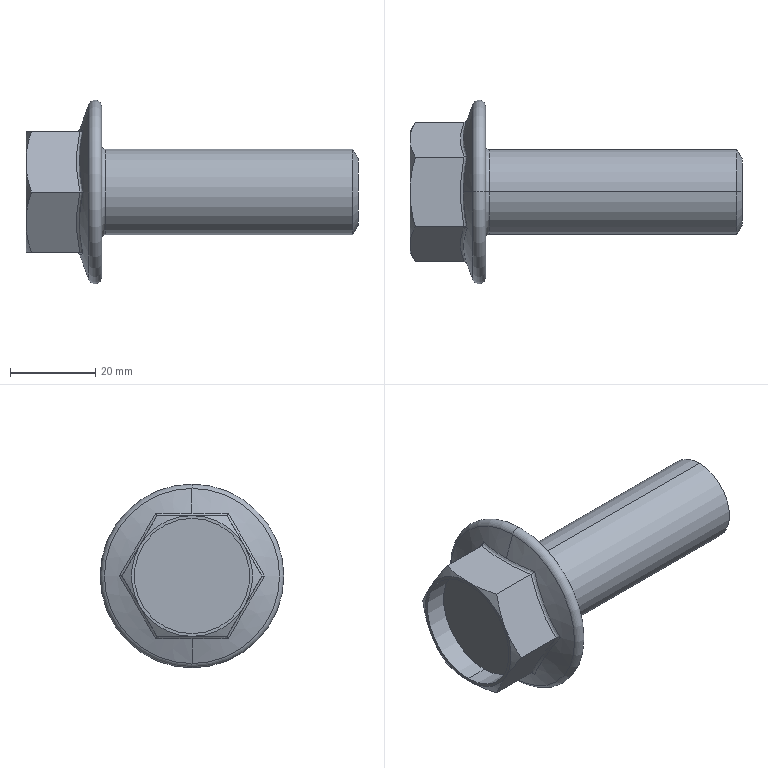Part | SolidWorks | 1 solid | 34 faces | box 77.7 x 43 x 43 mm | volume 30766 mm3 | cone 10 | plane 10 | spline 6 | torus 4 | cylinder 4 | commonest cylinder face diameters 20 x2 27 x2
STEP:
#1=CARTESIAN_POINT('',(0.,0.,-10.8));
#2=VERTEX_POINT('',#1);
#3=CARTESIAN_POINT('',(0.,0.,10.8));
#4=VERTEX_POINT('',#3);
#5=CARTESIAN_POINT('',(0.,0.,0.));
#6=DIRECTION('',(-1.,0.,0.));
#7=DIRECTION('',(0.,0.,1.));
#8=AXIS2_PLACEMENT_3D('',#5,#6,#7);
#9=CIRCLE('',#8,10.8);
#10=EDGE_CURVE('',#2,#4,#9,.T.);
#11=ORIENTED_EDGE('',*,*,#10,.F.);
#12=CARTESIAN_POINT('',(0.8,0.,-10.));
#13=VERTEX_POINT('',#12);
#14=CARTESIAN_POINT('',(0.8,0.,-10.8));
#15=DIRECTION('',(0.,1.,0.));
#16=DIRECTION('',(0.,0.,1.));
#17=AXIS2_PLACEMENT_3D('',#14,#15,#16);
#18=CIRCLE('',#17,0.8);
#19=EDGE_CURVE('',#2,#13,#18,.T.);
#20=ORIENTED_EDGE('',*,*,#19,.T.);
#21=CARTESIAN_POINT('',(0.8,0.,10.));
#22=VERTEX_POINT('',#21);
#23=CARTESIAN_POINT('',(0.8,0.,0.));
#24=DIRECTION('',(1.,0.,0.));
#25=DIRECTION('',(0.,0.,1.));
#26=AXIS2_PLACEMENT_3D('',#23,#24,#25);
#27=CIRCLE('',#26,10.);
#28=EDGE_CURVE('',#22,#13,#27,.T.);
#29=ORIENTED_EDGE('',*,*,#28,.F.);
#30=CARTESIAN_POINT('',(0.8,0.,10.8));
#31=DIRECTION('',(0.,-1.,0.));
#32=DIRECTION('',(0.,0.,-1.));
#33=AXIS2_PLACEMENT_3D('',#30,#31,#32);
#34=CIRCLE('',#33,0.8);
#35=EDGE_CURVE('',#4,#22,#34,.T.);
#36=ORIENTED_EDGE('',*,*,#35,.F.);
#37=EDGE_LOOP('',(#11,#20,#29,#36));
#38=FACE_OUTER_BOUND('',#37,.T.);
#39=CARTESIAN_POINT('',(0.8,0.,0.));
#40=DIRECTION('',(-1.,0.,0.));
#41=DIRECTION('',(0.,0.,1.));
#42=AXIS2_PLACEMENT_3D('',#39,#40,#41);
#43=TOROIDAL_SURFACE('',#42,10.8,0.8);
#44=ADVANCED_FACE('',(#38),#43,.F.);
#45=CARTESIAN_POINT('',(60.,0.,7.835));
#46=VERTEX_POINT('',#45);
#47=CARTESIAN_POINT('',(60.,0.,-7.835));
#48=VERTEX_POINT('',#47);
#49=CARTESIAN_POINT('',(60.,0.,0.));
#50=DIRECTION('',(-1.,0.,0.));
#51=DIRECTION('',(0.,0.,1.));
#52=AXIS2_PLACEMENT_3D('',#49,#50,#51);
#53=CIRCLE('',#52,7.835);
#54=EDGE_CURVE('',#46,#48,#53,.T.);
#55=ORIENTED_EDGE('',*,*,#54,.T.);
#56=CARTESIAN_POINT('',(58.75,0.,-10.));
#57=VERTEX_POINT('',#56);
#58=CARTESIAN_POINT('',(58.75,0.,-10.));
#59=DIRECTION('',(-0.5,0.,-0.866));
#60=VECTOR('',#59,1000.);
#61=LINE('',#58,#60);
#62=EDGE_CURVE('',#48,#57,#61,.T.);
#63=ORIENTED_EDGE('',*,*,#62,.T.);
#64=CARTESIAN_POINT('',(58.75,0.,10.));
#65=VERTEX_POINT('',#64);
#66=CARTESIAN_POINT('',(58.75,0.,0.));
#67=DIRECTION('',(-1.,0.,0.));
#68=DIRECTION('',(0.,0.,1.));
#69=AXIS2_PLACEMENT_3D('',#66,#67,#68);
#70=CIRCLE('',#69,10.);
#71=EDGE_CURVE('',#65,#57,#70,.T.);
#72=ORIENTED_EDGE('',*,*,#71,.F.);
#73=CARTESIAN_POINT('',(58.75,0.,10.));
#74=DIRECTION('',(-0.5,0.,0.866));
#75=VECTOR('',#74,1000.);
#76=LINE('',#73,#75);
#77=EDGE_CURVE('',#46,#65,#76,.T.);
#78=ORIENTED_EDGE('',*,*,#77,.F.);
#79=EDGE_LOOP('',(#55,#63,#72,#78));
#80=FACE_OUTER_BOUND('',#79,.T.);
#81=CARTESIAN_POINT('',(58.75,0.,0.));
#82=DIRECTION('',(-1.,0.,0.));
#83=DIRECTION('',(0.,0.,1.));
#84=AXIS2_PLACEMENT_3D('',#81,#82,#83);
#85=CONICAL_SURFACE('',#84,10.,1.047);
#86=ADVANCED_FACE('',(#80),#85,.T.);
#87=CARTESIAN_POINT('',(-12.411,0.,-13.5));
#88=VERTEX_POINT('',#87);
#89=CARTESIAN_POINT('',(-12.411,0.,13.5));
#90=VERTEX_POINT('',#89);
#91=CARTESIAN_POINT('',(-12.411,0.,0.));
#92=DIRECTION('',(-1.,0.,0.));
#93=DIRECTION('',(0.,0.,1.));
#94=AXIS2_PLACEMENT_3D('',#91,#92,#93);
#95=CIRCLE('',#94,13.5);
#96=EDGE_CURVE('',#88,#90,#95,.T.);
#97=ORIENTED_EDGE('',*,*,#96,.F.);
#98=CARTESIAN_POINT('',(-17.7,0.,-13.5));
#99=VERTEX_POINT('',#98);
#100=CARTESIAN_POINT('',(-12.411,0.,-13.5));
#101=DIRECTION('',(-1.,0.,0.));
#102=VECTOR('',#101,1000.);
#103=LINE('',#100,#102);
#104=EDGE_CURVE('',#88,#99,#103,.T.);
#105=ORIENTED_EDGE('',*,*,#104,.T.);
#106=CARTESIAN_POINT('',(-17.7,0.,13.5));
#107=VERTEX_POINT('',#106);
#108=CARTESIAN_POINT('',(-17.7,0.,0.));
#109=DIRECTION('',(-1.,0.,0.));
#110=DIRECTION('',(0.,0.,1.));
#111=AXIS2_PLACEMENT_3D('',#108,#109,#110);
#112=CIRCLE('',#111,13.5);
#113=EDGE_CURVE('',#99,#107,#112,.T.);
#114=ORIENTED_EDGE('',*,*,#113,.T.);
#115=CARTESIAN_POINT('',(-12.411,0.,13.5));
#116=DIRECTION('',(-1.,0.,0.));
#117=VECTOR('',#116,1000.);
#118=LINE('',#115,#117);
#119=EDGE_CURVE('',#90,#107,#118,.T.);
#120=ORIENTED_EDGE('',*,*,#119,.F.);
#121=EDGE_LOOP('',(#97,#105,#114,#120));
#122=FACE_OUTER_BOUND('',#121,.T.);
#123=CARTESIAN_POINT('',(-12.411,0.,0.));
#124=DIRECTION('',(-1.,0.,0.));
#125=DIRECTION('',(0.,0.,1.));
#126=AXIS2_PLACEMENT_3D('',#123,#124,#125);
#127=CYLINDRICAL_SURFACE('',#126,13.5);
#128=ADVANCED_FACE('',(#122),#127,.F.);
#129=CARTESIAN_POINT('',(0.,0.,19.953));
#130=VERTEX_POINT('',#129);
#131=CARTESIAN_POINT('',(0.,0.,-19.953));
#132=VERTEX_POINT('',#131);
#133=CARTESIAN_POINT('',(0.,0.,0.));
#134=DIRECTION('',(-1.,0.,0.));
#135=DIRECTION('',(0.,0.,1.));
#136=AXIS2_PLACEMENT_3D('',#133,#134,#135);
#137=CIRCLE('',#136,19.953);
#138=EDGE_CURVE('',#130,#132,#137,.T.);
#139=ORIENTED_EDGE('',*,*,#138,.T.);
#140=CARTESIAN_POINT('',(-3.,0.,-20.482));
#141=VERTEX_POINT('',#140);
#142=CARTESIAN_POINT('',(-1.547,0.,-19.953));
#143=DIRECTION('',(0.,1.,0.));
#144=DIRECTION('',(0.,0.,1.));
#145=AXIS2_PLACEMENT_3D('',#142,#143,#144);
#146=CIRCLE('',#145,1.547);
#147=EDGE_CURVE('',#132,#141,#146,.T.);
#148=ORIENTED_EDGE('',*,*,#147,.T.);
#149=CARTESIAN_POINT('',(-3.,0.,20.482));
#150=VERTEX_POINT('',#149);
#151=CARTESIAN_POINT('',(-3.,0.,0.));
#152=DIRECTION('',(-1.,0.,0.));
#153=DIRECTION('',(0.,0.,1.));
#154=AXIS2_PLACEMENT_3D('',#151,#152,#153);
#155=CIRCLE('',#154,20.482);
#156=EDGE_CURVE('',#150,#141,#155,.T.);
#157=ORIENTED_EDGE('',*,*,#156,.F.);
#158=CARTESIAN_POINT('',(-1.547,0.,19.953));
#159=DIRECTION('',(0.,-1.,0.));
#160=DIRECTION('',(0.,0.,-1.));
#161=AXIS2_PLACEMENT_3D('',#158,#159,#160);
#162=CIRCLE('',#161,1.547);
#163=EDGE_CURVE('',#130,#150,#162,.T.);
#164=ORIENTED_EDGE('',*,*,#163,.F.);
#165=EDGE_LOOP('',(#139,#148,#157,#164));
#166=FACE_OUTER_BOUND('',#165,.T.);
#167=CARTESIAN_POINT('',(-1.547,0.,0.));
#168=DIRECTION('',(-1.,0.,0.));
#169=DIRECTION('',(0.,0.,1.));
#170=AXIS2_PLACEMENT_3D('',#167,#168,#169);
#171=TOROIDAL_SURFACE('',#170,19.953,1.547);
#172=ADVANCED_FACE('',(#166),#171,.T.);
#173=CARTESIAN_POINT('',(-4.275,8.49,14.705));
#174=VERTEX_POINT('',#173);
#175=CARTESIAN_POINT('',(-5.116,0.,14.669));
#176=VERTEX_POINT('',#175);
#177=CARTESIAN_POINT('',(-4.275,8.49,14.705));
#178=CARTESIAN_POINT('',(-4.533,7.087,14.695));
#179=CARTESIAN_POINT('',(-4.745,5.679,14.686));
#180=CARTESIAN_POINT('',(-5.037,2.85,14.673));
#181=CARTESIAN_POINT('',(-5.116,1.429,14.669));
#182=CARTESIAN_POINT('',(-5.116,0.,14.669));
#183=B_SPLINE_CURVE_WITH_KNOTS('',3,(#177,#178,#179,#180,#181,#182),.UNSPECIFIED.,.F.,.F.,(4,2,4),(0.,0.004266,0.008532),.UNSPECIFIED.);
#184=EDGE_CURVE('',#174,#176,#183,.T.);
#185=ORIENTED_EDGE('',*,*,#184,.T.);
#186=CARTESIAN_POINT('',(-3.,0.,20.482));
#187=DIRECTION('',(0.342,0.,0.9397));
#188=VECTOR('',#187,1000.);
#189=LINE('',#186,#188);
#190=EDGE_CURVE('',#176,#150,#189,.T.);
#191=ORIENTED_EDGE('',*,*,#190,.T.);
#192=ORIENTED_EDGE('',*,*,#156,.T.);
#193=CARTESIAN_POINT('',(-5.116,0.,-14.669));
#194=VERTEX_POINT('',#193);
#195=CARTESIAN_POINT('',(-3.,0.,-20.482));
#196=DIRECTION('',(0.342,0.,-0.9397));
#197=VECTOR('',#196,1000.);
#198=LINE('',#195,#197);
#199=EDGE_CURVE('',#194,#141,#198,.T.);
#200=ORIENTED_EDGE('',*,*,#199,.F.);
#201=CARTESIAN_POINT('',(-4.275,8.49,-14.705));
#202=VERTEX_POINT('',#201);
#203=CARTESIAN_POINT('',(-5.116,0.,-14.669));
#204=CARTESIAN_POINT('',(-5.116,1.425,-14.669));
#205=CARTESIAN_POINT('',(-5.037,2.85,-14.673));
#206=CARTESIAN_POINT('',(-4.745,5.682,-14.686));
#207=CARTESIAN_POINT('',(-4.533,7.089,-14.695));
#208=CARTESIAN_POINT('',(-4.275,8.49,-14.705));
#209=B_SPLINE_CURVE_WITH_KNOTS('',3,(#203,#204,#205,#206,#207,#208),.UNSPECIFIED.,.F.,.F.,(4,2,4),(0.008532,0.01279,0.01704),.UNSPECIFIED.);
#210=EDGE_CURVE('',#194,#202,#209,.T.);
#211=ORIENTED_EDGE('',*,*,#210,.T.);
#212=CARTESIAN_POINT('',(-4.275,16.98,0.));
#213=VERTEX_POINT('',#212);
#214=CARTESIAN_POINT('',(-4.275,8.49,-14.705));
#215=CARTESIAN_POINT('',(-4.533,9.182,-13.487));
#216=CARTESIAN_POINT('',(-4.745,9.877,-12.264));
#217=CARTESIAN_POINT('',(-5.037,11.278,-9.811));
#218=CARTESIAN_POINT('',(-5.116,11.984,-8.579));
#219=CARTESIAN_POINT('',(-5.116,13.412,-6.108));
#220=CARTESIAN_POINT('',(-5.038,14.128,-4.874));
#221=CARTESIAN_POINT('',(-4.745,15.558,-2.426));
#222=CARTESIAN_POINT('',(-4.533,16.27,-1.21));
#223=CARTESIAN_POINT('',(-4.275,16.98,0.));
#224=B_SPLINE_CURVE_WITH_KNOTS('',3,(#214,#215,#216,#217,#218,#219,#220,#221,#222,#223),.UNSPECIFIED.,.F.,.F.,(4,2,2,2,4),(0.,0.004261,0.008521,0.01278,0.01704),.UNSPECIFIED.);
#225=EDGE_CURVE('',#202,#213,#224,.T.);
#226=ORIENTED_EDGE('',*,*,#225,.T.);
#227=CARTESIAN_POINT('',(-4.275,16.98,0.));
#228=CARTESIAN_POINT('',(-4.533,16.271,1.209));
#229=CARTESIAN_POINT('',(-4.745,15.56,2.422));
#230=CARTESIAN_POINT('',(-5.037,14.135,4.862));
#231=CARTESIAN_POINT('',(-5.116,13.422,6.089));
#232=CARTESIAN_POINT('',(-5.116,11.995,8.561));
#233=CARTESIAN_POINT('',(-5.038,11.285,9.798));
#234=CARTESIAN_POINT('',(-4.745,9.879,12.261));
#235=CARTESIAN_POINT('',(-4.533,9.183,13.485));
#236=CARTESIAN_POINT('',(-4.275,8.49,14.705));
#237=B_SPLINE_CURVE_WITH_KNOTS('',3,(#227,#228,#229,#230,#231,#232,#233,#234,#235,#236),.UNSPECIFIED.,.F.,.F.,(4,2,2,2,4),(0.,0.004261,0.008521,0.01278,0.01704),.UNSPECIFIED.);
#238=EDGE_CURVE('',#213,#174,#237,.T.);
#239=ORIENTED_EDGE('',*,*,#238,.T.);
#240=EDGE_LOOP('',(#185,#191,#192,#200,#211,#226,#239));
#241=FACE_OUTER_BOUND('',#240,.T.);
#242=CARTESIAN_POINT('',(-3.,0.,0.));
#243=DIRECTION('',(1.,0.,0.));
#244=DIRECTION('',(0.,0.,-1.));
#245=AXIS2_PLACEMENT_3D('',#242,#243,#244);
#246=CONICAL_SURFACE('',#245,20.482,1.222);
#247=ADVANCED_FACE('',(#241),#246,.T.);
#248=ORIENTED_EDGE('',*,*,#71,.T.);
#249=CARTESIAN_POINT('',(60.,0.,-10.));
#250=DIRECTION('',(-1.,0.,0.));
#251=VECTOR('',#250,1000.);
#252=LINE('',#249,#251);
#253=EDGE_CURVE('',#57,#13,#252,.T.);
#254=ORIENTED_EDGE('',*,*,#253,.T.);
#255=CARTESIAN_POINT('',(0.8,0.,0.));
#256=DIRECTION('',(1.,0.,0.));
#257=DIRECTION('',(0.,0.,1.));
#258=AXIS2_PLACEMENT_3D('',#255,#256,#257);
#259=CIRCLE('',#258,10.);
#260=EDGE_CURVE('',#13,#22,#259,.T.);
#261=ORIENTED_EDGE('',*,*,#260,.T.);
#262=CARTESIAN_POINT('',(60.,0.,10.));
#263=DIRECTION('',(-1.,0.,0.));
#264=VECTOR('',#263,1000.);
#265=LINE('',#262,#264);
#266=EDGE_CURVE('',#65,#22,#265,.T.);
#267=ORIENTED_EDGE('',*,*,#266,.F.);
#268=EDGE_LOOP('',(#248,#254,#261,#267));
#269=FACE_OUTER_BOUND('',#268,.T.);
#270=CARTESIAN_POINT('',(60.,0.,0.));
#271=DIRECTION('',(-1.,0.,0.));
#272=DIRECTION('',(0.,0.,1.));
#273=AXIS2_PLACEMENT_3D('',#270,#271,#272);
#274=CYLINDRICAL_SURFACE('',#273,10.);
#275=ADVANCED_FACE('',(#269),#274,.T.);
#276=ORIENTED_EDGE('',*,*,#253,.F.);
#277=CARTESIAN_POINT('',(58.75,0.,0.));
#278=DIRECTION('',(-1.,0.,0.));
#279=DIRECTION('',(0.,0.,1.));
#280=AXIS2_PLACEMENT_3D('',#277,#278,#279);
#281=CIRCLE('',#280,10.);
#282=EDGE_CURVE('',#57,#65,#281,.T.);
#283=ORIENTED_EDGE('',*,*,#282,.T.);
#284=ORIENTED_EDGE('',*,*,#266,.T.);
#285=ORIENTED_EDGE('',*,*,#28,.T.);
#286=EDGE_LOOP('',(#276,#283,#284,#285));
#287=FACE_OUTER_BOUND('',#286,.T.);
#288=CARTESIAN_POINT('',(60.,0.,0.));
#289=DIRECTION('',(-1.,0.,0.));
#290=DIRECTION('',(0.,0.,1.));
#291=AXIS2_PLACEMENT_3D('',#288,#289,#290);
#292=CYLINDRICAL_SURFACE('',#291,10.);
#293=ADVANCED_FACE('',(#287),#292,.T.);
#294=CARTESIAN_POINT('',(0.,0.,0.));
#295=DIRECTION('',(-1.,0.,0.));
#296=DIRECTION('',(0.,0.,1.));
#297=AXIS2_PLACEMENT_3D('',#294,#295,#296);
#298=CIRCLE('',#297,10.8);
#299=EDGE_CURVE('',#4,#2,#298,.T.);
#300=ORIENTED_EDGE('',*,*,#299,.T.);
#301=ORIENTED_EDGE('',*,*,#10,.T.);
#302=EDGE_LOOP('',(#300,#301));
#303=FACE_BOUND('',#302,.T.);
#304=ORIENTED_EDGE('',*,*,#138,.F.);
#305=CARTESIAN_POINT('',(0.,0.,0.));
#306=DIRECTION('',(-1.,0.,0.));
#307=DIRECTION('',(0.,0.,1.));
#308=AXIS2_PLACEMENT_3D('',#305,#306,#307);
#309=CIRCLE('',#308,19.953);
#310=EDGE_CURVE('',#132,#130,#309,.T.);
#311=ORIENTED_EDGE('',*,*,#310,.F.);
#312=EDGE_LOOP('',(#304,#311));
#313=FACE_OUTER_BOUND('',#312,.T.);
#314=CARTESIAN_POINT('',(0.,0.,0.));
#315=DIRECTION('',(-1.,0.,0.));
#316=DIRECTION('',(0.,0.,1.));
#317=AXIS2_PLACEMENT_3D('',#314,#315,#316);
#318=PLANE('',#317);
#319=ADVANCED_FACE('',(#303,#313),#318,.F.);
#320=CARTESIAN_POINT('',(-16.437,8.165,14.142));
#321=VERTEX_POINT('',#320);
#322=CARTESIAN_POINT('',(-5.109,8.165,14.142));
#323=VERTEX_POINT('',#322);
#324=CARTESIAN_POINT('',(-17.7,8.165,14.142));
#325=DIRECTION('',(1.,0.,0.));
#326=VECTOR('',#325,1000.);
#327=LINE('',#324,#326);
#328=EDGE_CURVE('',#321,#323,#327,.T.);
#329=ORIENTED_EDGE('',*,*,#328,.T.);
#330=CARTESIAN_POINT('',(-5.109,16.33,0.));
#331=VERTEX_POINT('',#330);
#332=CARTESIAN_POINT('',(-5.109,8.165,14.142));
#333=CARTESIAN_POINT('',(-5.345,8.84,12.972));
#334=CARTESIAN_POINT('',(-5.536,9.518,11.799));
#335=CARTESIAN_POINT('',(-5.798,10.878,9.443));
#336=CARTESIAN_POINT('',(-5.868,11.561,8.26));
#337=CARTESIAN_POINT('',(-5.868,12.934,5.882));
#338=CARTESIAN_POINT('',(-5.798,13.617,4.699));
#339=CARTESIAN_POINT('',(-5.536,14.977,2.343));
#340=CARTESIAN_POINT('',(-5.345,15.655,1.17));
#341=CARTESIAN_POINT('',(-5.109,16.33,0.));
#342=B_SPLINE_CURVE_WITH_KNOTS('',3,(#332,#333,#334,#335,#336,#337,#338,#339,#340,#341),.UNSPECIFIED.,.F.,.F.,(4,2,2,2,4),(0.,0.0041,0.0082,0.0123,0.0164),.UNSPECIFIED.);
#343=EDGE_CURVE('',#323,#331,#342,.T.);
#344=ORIENTED_EDGE('',*,*,#343,.T.);
#345=CARTESIAN_POINT('',(-16.437,16.33,0.));
#346=VERTEX_POINT('',#345);
#347=CARTESIAN_POINT('',(-17.7,16.33,0.));
#348=DIRECTION('',(1.,0.,0.));
#349=VECTOR('',#348,1000.);
#350=LINE('',#347,#349);
#351=EDGE_CURVE('',#346,#331,#350,.T.);
#352=ORIENTED_EDGE('',*,*,#351,.F.);
#353=CARTESIAN_POINT('',(-17.7,12.247,7.071));
#354=VERTEX_POINT('',#353);
#355=CARTESIAN_POINT('',(-17.7,12.247,7.071));
#356=CARTESIAN_POINT('',(-17.7,12.594,6.471));
#357=CARTESIAN_POINT('',(-17.67,12.942,5.868));
#358=CARTESIAN_POINT('',(-17.555,13.63,4.676));
#359=CARTESIAN_POINT('',(-17.469,13.972,4.084));
#360=CARTESIAN_POINT('',(-17.139,14.992,2.317));
#361=CARTESIAN_POINT('',(-16.821,15.664,1.154));
#362=CARTESIAN_POINT('',(-16.437,16.33,0.));
#363=B_SPLINE_CURVE_WITH_KNOTS('',3,(#355,#356,#357,#358,#359,#360,#361,#362),.UNSPECIFIED.,.F.,.F.,(4,2,2,4),(0.008262,0.01032,0.01238,0.01649),.UNSPECIFIED.);
#364=EDGE_CURVE('',#354,#346,#363,.T.);
#365=ORIENTED_EDGE('',*,*,#364,.F.);
#366=CARTESIAN_POINT('',(-16.437,8.165,14.142));
#367=CARTESIAN_POINT('',(-16.822,8.833,12.985));
#368=CARTESIAN_POINT('',(-17.14,9.506,11.82));
#369=CARTESIAN_POINT('',(-17.58,10.865,9.466));
#370=CARTESIAN_POINT('',(-17.7,11.552,8.276));
#371=CARTESIAN_POINT('',(-17.7,12.247,7.071));
#372=B_SPLINE_CURVE_WITH_KNOTS('',3,(#366,#367,#368,#369,#370,#371),.UNSPECIFIED.,.F.,.F.,(4,2,4),(0.000000238,0.004131,0.008262),.UNSPECIFIED.);
#373=EDGE_CURVE('',#321,#354,#372,.T.);
#374=ORIENTED_EDGE('',*,*,#373,.F.);
#375=EDGE_LOOP('',(#329,#344,#352,#365,#374));
#376=FACE_OUTER_BOUND('',#375,.T.);
#377=CARTESIAN_POINT('',(-17.7,8.165,14.142));
#378=DIRECTION('',(0.,-0.866,-0.5));
#379=DIRECTION('',(0.,0.5,-0.866));
#380=AXIS2_PLACEMENT_3D('',#377,#378,#379);
#381=PLANE('',#380);
#382=ADVANCED_FACE('',(#376),#381,.F.);
#383=ORIENTED_EDGE('',*,*,#351,.T.);
#384=CARTESIAN_POINT('',(-5.109,8.165,-14.142));
#385=VERTEX_POINT('',#384);
#386=CARTESIAN_POINT('',(-5.109,16.33,0.));
#387=CARTESIAN_POINT('',(-5.345,15.655,-1.17));
#388=CARTESIAN_POINT('',(-5.536,14.977,-2.343));
#389=CARTESIAN_POINT('',(-5.798,13.617,-4.699));
#390=CARTESIAN_POINT('',(-5.868,12.934,-5.882));
#391=CARTESIAN_POINT('',(-5.868,11.561,-8.26));
#392=CARTESIAN_POINT('',(-5.798,10.878,-9.443));
#393=CARTESIAN_POINT('',(-5.536,9.518,-11.799));
#394=CARTESIAN_POINT('',(-5.345,8.84,-12.972));
#395=CARTESIAN_POINT('',(-5.109,8.165,-14.142));
#396=B_SPLINE_CURVE_WITH_KNOTS('',3,(#386,#387,#388,#389,#390,#391,#392,#393,#394,#395),.UNSPECIFIED.,.F.,.F.,(4,2,2,2,4),(0.,0.0041,0.0082,0.0123,0.0164),.UNSPECIFIED.);
#397=EDGE_CURVE('',#331,#385,#396,.T.);
#398=ORIENTED_EDGE('',*,*,#397,.T.);
#399=CARTESIAN_POINT('',(-16.437,8.165,-14.142));
#400=VERTEX_POINT('',#399);
#401=CARTESIAN_POINT('',(-17.7,8.165,-14.142));
#402=DIRECTION('',(1.,0.,0.));
#403=VECTOR('',#402,1000.);
#404=LINE('',#401,#403);
#405=EDGE_CURVE('',#400,#385,#404,.T.);
#406=ORIENTED_EDGE('',*,*,#405,.F.);
#407=CARTESIAN_POINT('',(-17.7,12.247,-7.071));
#408=VERTEX_POINT('',#407);
#409=CARTESIAN_POINT('',(-17.7,12.247,-7.071));
#410=CARTESIAN_POINT('',(-17.7,11.901,-7.671));
#411=CARTESIAN_POINT('',(-17.67,11.553,-8.274));
#412=CARTESIAN_POINT('',(-17.555,10.865,-9.466));
#413=CARTESIAN_POINT('',(-17.469,10.523,-10.059));
#414=CARTESIAN_POINT('',(-17.139,9.503,-11.825));
#415=CARTESIAN_POINT('',(-16.821,8.831,-12.988));
#416=CARTESIAN_POINT('',(-16.437,8.165,-14.142));
#417=B_SPLINE_CURVE_WITH_KNOTS('',3,(#409,#410,#411,#412,#413,#414,#415,#416),.UNSPECIFIED.,.F.,.F.,(4,2,2,4),(0.008262,0.01032,0.01238,0.01649),.UNSPECIFIED.);
#418=EDGE_CURVE('',#408,#400,#417,.T.);
#419=ORIENTED_EDGE('',*,*,#418,.F.);
#420=CARTESIAN_POINT('',(-16.437,16.33,0.));
#421=CARTESIAN_POINT('',(-16.822,15.662,-1.157));
#422=CARTESIAN_POINT('',(-17.14,14.989,-2.322));
#423=CARTESIAN_POINT('',(-17.58,13.63,-4.677));
#424=CARTESIAN_POINT('',(-17.7,12.943,-5.866));
#425=CARTESIAN_POINT('',(-17.7,12.247,-7.071));
#426=B_SPLINE_CURVE_WITH_KNOTS('',3,(#420,#421,#422,#423,#424,#425),.UNSPECIFIED.,.F.,.F.,(4,2,4),(0.000000238,0.004131,0.008262),.UNSPECIFIED.);
#427=EDGE_CURVE('',#346,#408,#426,.T.);
#428=ORIENTED_EDGE('',*,*,#427,.F.);
#429=EDGE_LOOP('',(#383,#398,#406,#419,#428));
#430=FACE_OUTER_BOUND('',#429,.T.);
#431=CARTESIAN_POINT('',(-17.7,16.33,0.));
#432=DIRECTION('',(0.,-0.866,0.5));
#433=DIRECTION('',(0.,-0.5,-0.866));
#434=AXIS2_PLACEMENT_3D('',#431,#432,#433);
#435=PLANE('',#434);
#436=ADVANCED_FACE('',(#430),#435,.F.);
#437=ORIENTED_EDGE('',*,*,#405,.T.);
#438=CARTESIAN_POINT('',(-5.109,-8.165,-14.142));
#439=VERTEX_POINT('',#438);
#440=CARTESIAN_POINT('',(-5.109,8.165,-14.142));
#441=CARTESIAN_POINT('',(-5.345,6.814,-14.142));
#442=CARTESIAN_POINT('',(-5.536,5.459,-14.142));
#443=CARTESIAN_POINT('',(-5.798,2.739,-14.142));
#444=CARTESIAN_POINT('',(-5.868,1.372,-14.142));
#445=CARTESIAN_POINT('',(-5.868,-1.373,-14.142));
#446=CARTESIAN_POINT('',(-5.798,-2.739,-14.142));
#447=CARTESIAN_POINT('',(-5.536,-5.46,-14.142));
#448=CARTESIAN_POINT('',(-5.345,-6.814,-14.142));
#449=CARTESIAN_POINT('',(-5.109,-8.165,-14.142));
#450=B_SPLINE_CURVE_WITH_KNOTS('',3,(#440,#441,#442,#443,#444,#445,#446,#447,#448,#449),.UNSPECIFIED.,.F.,.F.,(4,2,2,2,4),(0.,0.0041,0.0082,0.0123,0.0164),.UNSPECIFIED.);
#451=EDGE_CURVE('',#385,#439,#450,.T.);
#452=ORIENTED_EDGE('',*,*,#451,.T.);
#453=CARTESIAN_POINT('',(-16.437,-8.165,-14.142));
#454=VERTEX_POINT('',#453);
#455=CARTESIAN_POINT('',(-17.7,-8.165,-14.142));
#456=DIRECTION('',(1.,0.,0.));
#457=VECTOR('',#456,1000.);
#458=LINE('',#455,#457);
#459=EDGE_CURVE('',#454,#439,#458,.T.);
#460=ORIENTED_EDGE('',*,*,#459,.F.);
#461=CARTESIAN_POINT('',(-17.7,0.,-14.142));
#462=VERTEX_POINT('',#461);
#463=CARTESIAN_POINT('',(-17.7,0.,-14.142));
#464=CARTESIAN_POINT('',(-17.7,-1.381,-14.142));
#465=CARTESIAN_POINT('',(-17.581,-2.752,-14.142));
#466=CARTESIAN_POINT('',(-17.142,-5.476,-14.142));
#467=CARTESIAN_POINT('',(-16.821,-6.836,-14.142));
#468=CARTESIAN_POINT('',(-16.437,-8.165,-14.142));
#469=B_SPLINE_CURVE_WITH_KNOTS('',3,(#463,#464,#465,#466,#467,#468),.UNSPECIFIED.,.F.,.F.,(4,2,4),(0.05501,0.05914,0.06328),.UNSPECIFIED.);
#470=EDGE_CURVE('',#462,#454,#469,.T.);
#471=ORIENTED_EDGE('',*,*,#470,.F.);
#472=CARTESIAN_POINT('',(-16.437,8.165,-14.142));
#473=CARTESIAN_POINT('',(-16.818,6.844,-14.142));
#474=CARTESIAN_POINT('',(-17.135,5.507,-14.142));
#475=CARTESIAN_POINT('',(-17.467,3.463,-14.142));
#476=CARTESIAN_POINT('',(-17.554,2.775,-14.142));
#477=CARTESIAN_POINT('',(-17.671,1.385,-14.142));
#478=CARTESIAN_POINT('',(-17.7,0.691,-14.142));
#479=CARTESIAN_POINT('',(-17.7,0.,-14.142));
#480=B_SPLINE_CURVE_WITH_KNOTS('',3,(#472,#473,#474,#475,#476,#477,#478,#479),.UNSPECIFIED.,.F.,.F.,(4,2,2,4),(0.04675,0.05088,0.05295,0.05501),.UNSPECIFIED.);
#481=EDGE_CURVE('',#400,#462,#480,.T.);
#482=ORIENTED_EDGE('',*,*,#481,.F.);
#483=EDGE_LOOP('',(#437,#452,#460,#471,#482));
#484=FACE_OUTER_BOUND('',#483,.T.);
#485=CARTESIAN_POINT('',(-17.7,8.165,-14.142));
#486=DIRECTION('',(0.,0.,1.));
#487=DIRECTION('',(0.,-1.,0.));
#488=AXIS2_PLACEMENT_3D('',#485,#486,#487);
#489=PLANE('',#488);
#490=ADVANCED_FACE('',(#484),#489,.F.);
#491=ORIENTED_EDGE('',*,*,#459,.T.);
#492=CARTESIAN_POINT('',(-5.109,-16.33,0.));
#493=VERTEX_POINT('',#492);
#494=CARTESIAN_POINT('',(-5.109,-8.165,-14.142));
#495=CARTESIAN_POINT('',(-5.345,-8.84,-12.972));
#496=CARTESIAN_POINT('',(-5.536,-9.518,-11.799));
#497=CARTESIAN_POINT('',(-5.798,-10.878,-9.443));
#498=CARTESIAN_POINT('',(-5.868,-11.561,-8.26));
#499=CARTESIAN_POINT('',(-5.868,-12.934,-5.882));
#500=CARTESIAN_POINT('',(-5.798,-13.617,-4.699));
#501=CARTESIAN_POINT('',(-5.536,-14.977,-2.343));
#502=CARTESIAN_POINT('',(-5.345,-15.655,-1.17));
#503=CARTESIAN_POINT('',(-5.109,-16.33,0.));
#504=B_SPLINE_CURVE_WITH_KNOTS('',3,(#494,#495,#496,#497,#498,#499,#500,#501,#502,#503),.UNSPECIFIED.,.F.,.F.,(4,2,2,2,4),(0.,0.0041,0.0082,0.0123,0.0164),.UNSPECIFIED.);
#505=EDGE_CURVE('',#439,#493,#504,.T.);
#506=ORIENTED_EDGE('',*,*,#505,.T.);
#507=CARTESIAN_POINT('',(-16.437,-16.33,0.));
#508=VERTEX_POINT('',#507);
#509=CARTESIAN_POINT('',(-17.7,-16.33,0.));
#510=DIRECTION('',(1.,0.,0.));
#511=VECTOR('',#510,1000.);
#512=LINE('',#509,#511);
#513=EDGE_CURVE('',#508,#493,#512,.T.);
#514=ORIENTED_EDGE('',*,*,#513,.F.);
#515=CARTESIAN_POINT('',(-17.7,-12.247,-7.071));
#516=VERTEX_POINT('',#515);
#517=CARTESIAN_POINT('',(-17.7,-12.247,-7.071));
#518=CARTESIAN_POINT('',(-17.7,-12.594,-6.471));
#519=CARTESIAN_POINT('',(-17.67,-12.942,-5.868));
#520=CARTESIAN_POINT('',(-17.555,-13.63,-4.676));
#521=CARTESIAN_POINT('',(-17.469,-13.972,-4.084));
#522=CARTESIAN_POINT('',(-17.139,-14.992,-2.317));
#523=CARTESIAN_POINT('',(-16.821,-15.664,-1.154));
#524=CARTESIAN_POINT('',(-16.437,-16.33,0.));
#525=B_SPLINE_CURVE_WITH_KNOTS('',3,(#517,#518,#519,#520,#521,#522,#523,#524),.UNSPECIFIED.,.F.,.F.,(4,2,2,4),(0.008262,0.01032,0.01238,0.01649),.UNSPECIFIED.);
#526=EDGE_CURVE('',#516,#508,#525,.T.);
#527=ORIENTED_EDGE('',*,*,#526,.F.);
#528=CARTESIAN_POINT('',(-16.437,-8.165,-14.142));
#529=CARTESIAN_POINT('',(-16.822,-8.833,-12.985));
#530=CARTESIAN_POINT('',(-17.14,-9.506,-11.82));
#531=CARTESIAN_POINT('',(-17.58,-10.865,-9.466));
#532=CARTESIAN_POINT('',(-17.7,-11.552,-8.276));
#533=CARTESIAN_POINT('',(-17.7,-12.247,-7.071));
#534=B_SPLINE_CURVE_WITH_KNOTS('',3,(#528,#529,#530,#531,#532,#533),.UNSPECIFIED.,.F.,.F.,(4,2,4),(0.000000238,0.004131,0.008262),.UNSPECIFIED.);
#535=EDGE_CURVE('',#454,#516,#534,.T.);
#536=ORIENTED_EDGE('',*,*,#535,.F.);
#537=EDGE_LOOP('',(#491,#506,#514,#527,#536));
#538=FACE_OUTER_BOUND('',#537,.T.);
#539=CARTESIAN_POINT('',(-17.7,-8.165,-14.142));
#540=DIRECTION('',(0.,0.866,0.5));
#541=DIRECTION('',(0.,-0.5,0.866));
#542=AXIS2_PLACEMENT_3D('',#539,#540,#541);
#543=PLANE('',#542);
#544=ADVANCED_FACE('',(#538),#543,.F.);
#545=ORIENTED_EDGE('',*,*,#513,.T.);
#546=CARTESIAN_POINT('',(-5.109,-8.165,14.142));
#547=VERTEX_POINT('',#546);
#548=CARTESIAN_POINT('',(-5.109,-16.33,0.));
#549=CARTESIAN_POINT('',(-5.345,-15.655,1.17));
#550=CARTESIAN_POINT('',(-5.536,-14.977,2.343));
#551=CARTESIAN_POINT('',(-5.798,-13.617,4.699));
#552=CARTESIAN_POINT('',(-5.868,-12.934,5.882));
#553=CARTESIAN_POINT('',(-5.868,-11.561,8.26));
#554=CARTESIAN_POINT('',(-5.798,-10.878,9.443));
#555=CARTESIAN_POINT('',(-5.536,-9.518,11.799));
#556=CARTESIAN_POINT('',(-5.345,-8.84,12.972));
#557=CARTESIAN_POINT('',(-5.109,-8.165,14.142));
#558=B_SPLINE_CURVE_WITH_KNOTS('',3,(#548,#549,#550,#551,#552,#553,#554,#555,#556,#557),.UNSPECIFIED.,.F.,.F.,(4,2,2,2,4),(0.,0.0041,0.0082,0.0123,0.0164),.UNSPECIFIED.);
#559=EDGE_CURVE('',#493,#547,#558,.T.);
#560=ORIENTED_EDGE('',*,*,#559,.T.);
#561=CARTESIAN_POINT('',(-16.437,-8.165,14.142));
#562=VERTEX_POINT('',#561);
#563=CARTESIAN_POINT('',(-17.7,-8.165,14.142));
#564=DIRECTION('',(1.,0.,0.));
#565=VECTOR('',#564,1000.);
#566=LINE('',#563,#565);
#567=EDGE_CURVE('',#562,#547,#566,.T.);
#568=ORIENTED_EDGE('',*,*,#567,.F.);
#569=CARTESIAN_POINT('',(-17.7,-12.247,7.071));
#570=VERTEX_POINT('',#569);
#571=CARTESIAN_POINT('',(-17.7,-12.247,7.071));
#572=CARTESIAN_POINT('',(-17.7,-11.901,7.671));
#573=CARTESIAN_POINT('',(-17.67,-11.553,8.274));
#574=CARTESIAN_POINT('',(-17.555,-10.865,9.466));
#575=CARTESIAN_POINT('',(-17.469,-10.523,10.059));
#576=CARTESIAN_POINT('',(-17.139,-9.503,11.825));
#577=CARTESIAN_POINT('',(-16.821,-8.831,12.988));
#578=CARTESIAN_POINT('',(-16.437,-8.165,14.142));
#579=B_SPLINE_CURVE_WITH_KNOTS('',3,(#571,#572,#573,#574,#575,#576,#577,#578),.UNSPECIFIED.,.F.,.F.,(4,2,2,4),(0.008262,0.01032,0.01238,0.01649),.UNSPECIFIED.);
#580=EDGE_CURVE('',#570,#562,#579,.T.);
#581=ORIENTED_EDGE('',*,*,#580,.F.);
#582=CARTESIAN_POINT('',(-16.437,-16.33,0.));
#583=CARTESIAN_POINT('',(-16.822,-15.662,1.157));
#584=CARTESIAN_POINT('',(-17.14,-14.989,2.322));
#585=CARTESIAN_POINT('',(-17.58,-13.63,4.677));
#586=CARTESIAN_POINT('',(-17.7,-12.943,5.866));
#587=CARTESIAN_POINT('',(-17.7,-12.247,7.071));
#588=B_SPLINE_CURVE_WITH_KNOTS('',3,(#582,#583,#584,#585,#586,#587),.UNSPECIFIED.,.F.,.F.,(4,2,4),(0.000000238,0.004131,0.008262),.UNSPECIFIED.);
#589=EDGE_CURVE('',#508,#570,#588,.T.);
#590=ORIENTED_EDGE('',*,*,#589,.F.);
#591=EDGE_LOOP('',(#545,#560,#568,#581,#590));
#592=FACE_OUTER_BOUND('',#591,.T.);
#593=CARTESIAN_POINT('',(-17.7,-16.33,0.));
#594=DIRECTION('',(0.,0.866,-0.5));
#595=DIRECTION('',(0.,0.5,0.866));
#596=AXIS2_PLACEMENT_3D('',#593,#594,#595);
#597=PLANE('',#596);
#598=ADVANCED_FACE('',(#592),#597,.F.);
#599=ORIENTED_EDGE('',*,*,#567,.T.);
#600=CARTESIAN_POINT('',(-5.109,-8.165,14.142));
#601=CARTESIAN_POINT('',(-5.345,-6.814,14.142));
#602=CARTESIAN_POINT('',(-5.536,-5.46,14.142));
#603=CARTESIAN_POINT('',(-5.798,-2.739,14.142));
#604=CARTESIAN_POINT('',(-5.868,-1.373,14.142));
#605=CARTESIAN_POINT('',(-5.868,1.372,14.142));
#606=CARTESIAN_POINT('',(-5.798,2.739,14.142));
#607=CARTESIAN_POINT('',(-5.536,5.459,14.142));
#608=CARTESIAN_POINT('',(-5.345,6.814,14.142));
#609=CARTESIAN_POINT('',(-5.109,8.165,14.142));
#610=B_SPLINE_CURVE_WITH_KNOTS('',3,(#600,#601,#602,#603,#604,#605,#606,#607,#608,#609),.UNSPECIFIED.,.F.,.F.,(4,2,2,2,4),(0.,0.0041,0.0082,0.0123,0.0164),.UNSPECIFIED.);
#611=EDGE_CURVE('',#547,#323,#610,.T.);
#612=ORIENTED_EDGE('',*,*,#611,.T.);
#613=ORIENTED_EDGE('',*,*,#328,.F.);
#614=CARTESIAN_POINT('',(-17.7,0.,14.142));
#615=VERTEX_POINT('',#614);
#616=CARTESIAN_POINT('',(-17.7,0.,14.142));
#617=CARTESIAN_POINT('',(-17.7,0.691,14.142));
#618=CARTESIAN_POINT('',(-17.671,1.385,14.142));
#619=CARTESIAN_POINT('',(-17.554,2.775,14.142));
#620=CARTESIAN_POINT('',(-17.467,3.463,14.142));
#621=CARTESIAN_POINT('',(-17.135,5.507,14.142));
#622=CARTESIAN_POINT('',(-16.818,6.844,14.142));
#623=CARTESIAN_POINT('',(-16.437,8.165,14.142));
#624=B_SPLINE_CURVE_WITH_KNOTS('',3,(#616,#617,#618,#619,#620,#621,#622,#623),.UNSPECIFIED.,.F.,.F.,(4,2,2,4),(0.02324,0.0253,0.02737,0.03151),.UNSPECIFIED.);
#625=EDGE_CURVE('',#615,#321,#624,.T.);
#626=ORIENTED_EDGE('',*,*,#625,.F.);
#627=CARTESIAN_POINT('',(-16.437,-8.165,14.142));
#628=CARTESIAN_POINT('',(-16.821,-6.836,14.142));
#629=CARTESIAN_POINT('',(-17.142,-5.476,14.142));
#630=CARTESIAN_POINT('',(-17.581,-2.752,14.142));
#631=CARTESIAN_POINT('',(-17.7,-1.381,14.142));
#632=CARTESIAN_POINT('',(-17.7,0.,14.142));
#633=B_SPLINE_CURVE_WITH_KNOTS('',3,(#627,#628,#629,#630,#631,#632),.UNSPECIFIED.,.F.,.F.,(4,2,4),(0.01497,0.0191,0.02324),.UNSPECIFIED.);
#634=EDGE_CURVE('',#562,#615,#633,.T.);
#635=ORIENTED_EDGE('',*,*,#634,.F.);
#636=EDGE_LOOP('',(#599,#612,#613,#626,#635));
#637=FACE_OUTER_BOUND('',#636,.T.);
#638=CARTESIAN_POINT('',(-17.7,-8.165,14.142));
#639=DIRECTION('',(0.,0.,-1.));
#640=DIRECTION('',(0.,1.,0.));
#641=AXIS2_PLACEMENT_3D('',#638,#639,#640);
#642=PLANE('',#641);
#643=ADVANCED_FACE('',(#637),#642,.F.);
#644=ORIENTED_EDGE('',*,*,#190,.F.);
#645=CARTESIAN_POINT('',(-4.275,-8.49,14.705));
#646=VERTEX_POINT('',#645);
#647=CARTESIAN_POINT('',(-5.116,0.,14.669));
#648=CARTESIAN_POINT('',(-5.116,-1.425,14.669));
#649=CARTESIAN_POINT('',(-5.037,-2.85,14.673));
#650=CARTESIAN_POINT('',(-4.745,-5.682,14.686));
#651=CARTESIAN_POINT('',(-4.533,-7.089,14.695));
#652=CARTESIAN_POINT('',(-4.275,-8.49,14.705));
#653=B_SPLINE_CURVE_WITH_KNOTS('',3,(#647,#648,#649,#650,#651,#652),.UNSPECIFIED.,.F.,.F.,(4,2,4),(0.008532,0.01279,0.01704),.UNSPECIFIED.);
#654=EDGE_CURVE('',#176,#646,#653,.T.);
#655=ORIENTED_EDGE('',*,*,#654,.T.);
#656=CARTESIAN_POINT('',(-4.275,-16.98,0.));
#657=VERTEX_POINT('',#656);
#658=CARTESIAN_POINT('',(-4.275,-8.49,14.705));
#659=CARTESIAN_POINT('',(-4.533,-9.182,13.487));
#660=CARTESIAN_POINT('',(-4.745,-9.877,12.264));
#661=CARTESIAN_POINT('',(-5.037,-11.278,9.811));
#662=CARTESIAN_POINT('',(-5.116,-11.984,8.579));
#663=CARTESIAN_POINT('',(-5.116,-13.412,6.108));
#664=CARTESIAN_POINT('',(-5.038,-14.128,4.874));
#665=CARTESIAN_POINT('',(-4.745,-15.558,2.426));
#666=CARTESIAN_POINT('',(-4.533,-16.27,1.21));
#667=CARTESIAN_POINT('',(-4.275,-16.98,0.));
#668=B_SPLINE_CURVE_WITH_KNOTS('',3,(#658,#659,#660,#661,#662,#663,#664,#665,#666,#667),.UNSPECIFIED.,.F.,.F.,(4,2,2,2,4),(0.,0.004261,0.008521,0.01278,0.01704),.UNSPECIFIED.);
#669=EDGE_CURVE('',#646,#657,#668,.T.);
#670=ORIENTED_EDGE('',*,*,#669,.T.);
#671=CARTESIAN_POINT('',(-4.275,-8.49,-14.705));
#672=VERTEX_POINT('',#671);
#673=CARTESIAN_POINT('',(-4.275,-16.98,0.));
#674=CARTESIAN_POINT('',(-4.533,-16.271,-1.209));
#675=CARTESIAN_POINT('',(-4.745,-15.56,-2.422));
#676=CARTESIAN_POINT('',(-5.037,-14.135,-4.862));
#677=CARTESIAN_POINT('',(-5.116,-13.422,-6.089));
#678=CARTESIAN_POINT('',(-5.116,-11.995,-8.561));
#679=CARTESIAN_POINT('',(-5.038,-11.285,-9.798));
#680=CARTESIAN_POINT('',(-4.745,-9.879,-12.261));
#681=CARTESIAN_POINT('',(-4.533,-9.183,-13.485));
#682=CARTESIAN_POINT('',(-4.275,-8.49,-14.705));
#683=B_SPLINE_CURVE_WITH_KNOTS('',3,(#673,#674,#675,#676,#677,#678,#679,#680,#681,#682),.UNSPECIFIED.,.F.,.F.,(4,2,2,2,4),(0.,0.004261,0.008521,0.01278,0.01704),.UNSPECIFIED.);
#684=EDGE_CURVE('',#657,#672,#683,.T.);
#685=ORIENTED_EDGE('',*,*,#684,.T.);
#686=CARTESIAN_POINT('',(-4.275,-8.49,-14.705));
#687=CARTESIAN_POINT('',(-4.533,-7.087,-14.695));
#688=CARTESIAN_POINT('',(-4.745,-5.679,-14.686));
#689=CARTESIAN_POINT('',(-5.037,-2.85,-14.673));
#690=CARTESIAN_POINT('',(-5.116,-1.429,-14.669));
#691=CARTESIAN_POINT('',(-5.116,0.,-14.669));
#692=B_SPLINE_CURVE_WITH_KNOTS('',3,(#686,#687,#688,#689,#690,#691),.UNSPECIFIED.,.F.,.F.,(4,2,4),(0.,0.004266,0.008532),.UNSPECIFIED.);
#693=EDGE_CURVE('',#672,#194,#692,.T.);
#694=ORIENTED_EDGE('',*,*,#693,.T.);
#695=ORIENTED_EDGE('',*,*,#199,.T.);
#696=CARTESIAN_POINT('',(-3.,0.,0.));
#697=DIRECTION('',(-1.,0.,0.));
#698=DIRECTION('',(0.,0.,1.));
#699=AXIS2_PLACEMENT_3D('',#696,#697,#698);
#700=CIRCLE('',#699,20.482);
#701=EDGE_CURVE('',#141,#150,#700,.T.);
#702=ORIENTED_EDGE('',*,*,#701,.T.);
#703=EDGE_LOOP('',(#644,#655,#670,#685,#694,#695,#702));
#704=FACE_OUTER_BOUND('',#703,.T.);
#705=CARTESIAN_POINT('',(-3.,0.,0.));
#706=DIRECTION('',(1.,0.,0.));
#707=DIRECTION('',(0.,0.,-1.));
#708=AXIS2_PLACEMENT_3D('',#705,#706,#707);
#709=CONICAL_SURFACE('',#708,20.482,1.222);
#710=ADVANCED_FACE('',(#704),#709,.T.);
#711=ORIENTED_EDGE('',*,*,#147,.F.);
#712=ORIENTED_EDGE('',*,*,#310,.T.);
#713=ORIENTED_EDGE('',*,*,#163,.T.);
#714=ORIENTED_EDGE('',*,*,#701,.F.);
#715=EDGE_LOOP('',(#711,#712,#713,#714));
#716=FACE_OUTER_BOUND('',#715,.T.);
#717=CARTESIAN_POINT('',(-1.547,0.,0.));
#718=DIRECTION('',(-1.,0.,0.));
#719=DIRECTION('',(0.,0.,1.));
#720=AXIS2_PLACEMENT_3D('',#717,#718,#719);
#721=TOROIDAL_SURFACE('',#720,19.953,1.547);
#722=ADVANCED_FACE('',(#716),#721,.T.);
#723=ORIENTED_EDGE('',*,*,#580,.T.);
#724=ORIENTED_EDGE('',*,*,#634,.T.);
#725=CARTESIAN_POINT('',(-17.7,0.,0.));
#726=DIRECTION('',(-1.,0.,0.));
#727=DIRECTION('',(0.,0.,1.));
#728=AXIS2_PLACEMENT_3D('',#725,#726,#727);
#729=CIRCLE('',#728,14.142);
#730=EDGE_CURVE('',#570,#615,#729,.T.);
#731=ORIENTED_EDGE('',*,*,#730,.F.);
#732=EDGE_LOOP('',(#723,#724,#731));
#733=FACE_OUTER_BOUND('',#732,.T.);
#734=CARTESIAN_POINT('',(-17.7,0.,0.));
#735=DIRECTION('',(1.,0.,0.));
#736=DIRECTION('',(0.,0.,1.));
#737=AXIS2_PLACEMENT_3D('',#734,#735,#736);
#738=CONICAL_SURFACE('',#737,14.142,1.047);
#739=ADVANCED_FACE('',(#733),#738,.T.);
#740=ORIENTED_EDGE('',*,*,#526,.T.);
#741=ORIENTED_EDGE('',*,*,#589,.T.);
#742=CARTESIAN_POINT('',(-17.7,0.,0.));
#743=DIRECTION('',(-1.,0.,0.));
#744=DIRECTION('',(0.,0.,1.));
#745=AXIS2_PLACEMENT_3D('',#742,#743,#744);
#746=CIRCLE('',#745,14.142);
#747=EDGE_CURVE('',#516,#570,#746,.T.);
#748=ORIENTED_EDGE('',*,*,#747,.F.);
#749=EDGE_LOOP('',(#740,#741,#748));
#750=FACE_OUTER_BOUND('',#749,.T.);
#751=CARTESIAN_POINT('',(-17.7,0.,0.));
#752=DIRECTION('',(1.,0.,0.));
#753=DIRECTION('',(0.,0.,1.));
#754=AXIS2_PLACEMENT_3D('',#751,#752,#753);
#755=CONICAL_SURFACE('',#754,14.142,1.047);
#756=ADVANCED_FACE('',(#750),#755,.T.);
#757=ORIENTED_EDGE('',*,*,#470,.T.);
#758=ORIENTED_EDGE('',*,*,#535,.T.);
#759=CARTESIAN_POINT('',(-17.7,0.,0.));
#760=DIRECTION('',(-1.,0.,0.));
#761=DIRECTION('',(0.,0.,1.));
#762=AXIS2_PLACEMENT_3D('',#759,#760,#761);
#763=CIRCLE('',#762,14.142);
#764=EDGE_CURVE('',#462,#516,#763,.T.);
#765=ORIENTED_EDGE('',*,*,#764,.F.);
#766=EDGE_LOOP('',(#757,#758,#765));
#767=FACE_OUTER_BOUND('',#766,.T.);
#768=CARTESIAN_POINT('',(-17.7,0.,0.));
#769=DIRECTION('',(1.,0.,0.));
#770=DIRECTION('',(0.,0.,1.));
#771=AXIS2_PLACEMENT_3D('',#768,#769,#770);
#772=CONICAL_SURFACE('',#771,14.142,1.047);
#773=ADVANCED_FACE('',(#767),#772,.T.);
#774=ORIENTED_EDGE('',*,*,#418,.T.);
#775=ORIENTED_EDGE('',*,*,#481,.T.);
#776=CARTESIAN_POINT('',(-17.7,0.,0.));
#777=DIRECTION('',(-1.,0.,0.));
#778=DIRECTION('',(0.,0.,1.));
#779=AXIS2_PLACEMENT_3D('',#776,#777,#778);
#780=CIRCLE('',#779,14.142);
#781=EDGE_CURVE('',#408,#462,#780,.T.);
#782=ORIENTED_EDGE('',*,*,#781,.F.);
#783=EDGE_LOOP('',(#774,#775,#782));
#784=FACE_OUTER_BOUND('',#783,.T.);
#785=CARTESIAN_POINT('',(-17.7,0.,0.));
#786=DIRECTION('',(1.,0.,0.));
#787=DIRECTION('',(0.,0.,1.));
#788=AXIS2_PLACEMENT_3D('',#785,#786,#787);
#789=CONICAL_SURFACE('',#788,14.142,1.047);
#790=ADVANCED_FACE('',(#784),#789,.T.);
#791=ORIENTED_EDGE('',*,*,#364,.T.);
#792=ORIENTED_EDGE('',*,*,#427,.T.);
#793=CARTESIAN_POINT('',(-17.7,0.,0.));
#794=DIRECTION('',(-1.,0.,0.));
#795=DIRECTION('',(0.,0.,1.));
#796=AXIS2_PLACEMENT_3D('',#793,#794,#795);
#797=CIRCLE('',#796,14.142);
#798=EDGE_CURVE('',#354,#408,#797,.T.);
#799=ORIENTED_EDGE('',*,*,#798,.F.);
#800=EDGE_LOOP('',(#791,#792,#799));
#801=FACE_OUTER_BOUND('',#800,.T.);
#802=CARTESIAN_POINT('',(-17.7,0.,0.));
#803=DIRECTION('',(1.,0.,0.));
#804=DIRECTION('',(0.,0.,1.));
#805=AXIS2_PLACEMENT_3D('',#802,#803,#804);
#806=CONICAL_SURFACE('',#805,14.142,1.047);
#807=ADVANCED_FACE('',(#801),#806,.T.);
#808=ORIENTED_EDGE('',*,*,#373,.T.);
#809=CARTESIAN_POINT('',(-17.7,0.,0.));
#810=DIRECTION('',(-1.,0.,0.));
#811=DIRECTION('',(0.,0.,1.));
#812=AXIS2_PLACEMENT_3D('',#809,#810,#811);
#813=CIRCLE('',#812,14.142);
#814=EDGE_CURVE('',#615,#354,#813,.T.);
#815=ORIENTED_EDGE('',*,*,#814,.F.);
#816=ORIENTED_EDGE('',*,*,#625,.T.);
#817=EDGE_LOOP('',(#808,#815,#816));
#818=FACE_OUTER_BOUND('',#817,.T.);
#819=CARTESIAN_POINT('',(-17.7,0.,0.));
#820=DIRECTION('',(1.,0.,0.));
#821=DIRECTION('',(0.,0.,1.));
#822=AXIS2_PLACEMENT_3D('',#819,#820,#821);
#823=CONICAL_SURFACE('',#822,14.142,1.047);
#824=ADVANCED_FACE('',(#818),#823,.T.);
#825=CARTESIAN_POINT('',(-17.7,0.,0.));
#826=DIRECTION('',(-1.,0.,0.));
#827=DIRECTION('',(0.,0.,1.));
#828=AXIS2_PLACEMENT_3D('',#825,#826,#827);
#829=CIRCLE('',#828,13.5);
#830=EDGE_CURVE('',#107,#99,#829,.T.);
#831=ORIENTED_EDGE('',*,*,#830,.F.);
#832=ORIENTED_EDGE('',*,*,#113,.F.);
#833=EDGE_LOOP('',(#831,#832));
#834=FACE_BOUND('',#833,.T.);
#835=ORIENTED_EDGE('',*,*,#730,.T.);
#836=ORIENTED_EDGE('',*,*,#814,.T.);
#837=ORIENTED_EDGE('',*,*,#798,.T.);
#838=ORIENTED_EDGE('',*,*,#781,.T.);
#839=ORIENTED_EDGE('',*,*,#764,.T.);
#840=ORIENTED_EDGE('',*,*,#747,.T.);
#841=EDGE_LOOP('',(#835,#836,#837,#838,#839,#840));
#842=FACE_OUTER_BOUND('',#841,.T.);
#843=CARTESIAN_POINT('',(-17.7,24.495,-14.142));
#844=DIRECTION('',(-1.,0.,0.));
#845=DIRECTION('',(0.,0.,1.));
#846=AXIS2_PLACEMENT_3D('',#843,#844,#845);
#847=PLANE('',#846);
#848=ADVANCED_FACE('',(#834,#842),#847,.T.);
#849=CARTESIAN_POINT('',(-4.275,-16.98,0.));
#850=CARTESIAN_POINT('',(-4.339,-16.804,0.));
#851=CARTESIAN_POINT('',(-4.448,-16.644,0.));
#852=CARTESIAN_POINT('',(-4.738,-16.405,0.));
#853=CARTESIAN_POINT('',(-4.919,-16.33,0.));
#854=CARTESIAN_POINT('',(-5.109,-16.33,0.));
#855=B_SPLINE_CURVE_WITH_KNOTS('',3,(#849,#850,#851,#852,#853,#854),.UNSPECIFIED.,.F.,.F.,(4,2,4),(-0.000005955,0.0005549,0.001116),.UNSPECIFIED.);
#856=EDGE_CURVE('',#657,#493,#855,.T.);
#857=ORIENTED_EDGE('',*,*,#856,.F.);
#858=ORIENTED_EDGE('',*,*,#669,.F.);
#859=CARTESIAN_POINT('',(-5.109,-8.165,14.142));
#860=CARTESIAN_POINT('',(-4.919,-8.165,14.142));
#861=CARTESIAN_POINT('',(-4.738,-8.203,14.207));
#862=CARTESIAN_POINT('',(-4.448,-8.322,14.414));
#863=CARTESIAN_POINT('',(-4.338,-8.403,14.554));
#864=CARTESIAN_POINT('',(-4.275,-8.49,14.705));
#865=B_SPLINE_CURVE_WITH_KNOTS('',3,(#859,#860,#861,#862,#863,#864),.UNSPECIFIED.,.F.,.F.,(4,2,4),(0.,0.0005589,0.001118),.UNSPECIFIED.);
#866=EDGE_CURVE('',#547,#646,#865,.T.);
#867=ORIENTED_EDGE('',*,*,#866,.F.);
#868=ORIENTED_EDGE('',*,*,#559,.F.);
#869=EDGE_LOOP('',(#857,#858,#867,#868));
#870=FACE_OUTER_BOUND('',#869,.T.);
#871=CARTESIAN_POINT('',(-4.256,-8.441,14.791));
#872=CARTESIAN_POINT('',(-4.428,-7.937,14.537));
#873=CARTESIAN_POINT('',(-5.008,-7.884,14.629));
#874=CARTESIAN_POINT('',(-4.515,-9.129,13.58));
#875=CARTESIAN_POINT('',(-4.691,-8.632,13.334));
#876=CARTESIAN_POINT('',(-5.267,-8.589,13.408));
#877=CARTESIAN_POINT('',(-4.73,-9.823,12.361));
#878=CARTESIAN_POINT('',(-4.911,-9.336,12.114));
#879=CARTESIAN_POINT('',(-5.482,-9.3,12.176));
#880=CARTESIAN_POINT('',(-5.03,-11.23,9.896));
#881=CARTESIAN_POINT('',(-5.218,-10.761,9.647));
#882=CARTESIAN_POINT('',(-5.781,-10.742,9.678));
#883=CARTESIAN_POINT('',(-5.114,-11.944,8.651));
#884=CARTESIAN_POINT('',(-5.305,-11.484,8.394));
#885=CARTESIAN_POINT('',(-5.866,-11.473,8.412));
#886=CARTESIAN_POINT('',(-5.118,-13.403,6.123));
#887=CARTESIAN_POINT('',(-5.31,-12.95,5.854));
#888=CARTESIAN_POINT('',(-5.87,-12.96,5.837));
#889=CARTESIAN_POINT('',(-5.038,-14.131,4.87));
#890=CARTESIAN_POINT('',(-5.227,-13.681,4.589));
#891=CARTESIAN_POINT('',(-5.79,-13.698,4.559));
#892=CARTESIAN_POINT('',(-4.739,-15.583,2.382));
#893=CARTESIAN_POINT('',(-4.921,-15.127,2.084));
#894=CARTESIAN_POINT('',(-5.491,-15.162,2.023));
#895=CARTESIAN_POINT('',(-4.521,-16.308,1.145));
#896=CARTESIAN_POINT('',(-4.697,-15.846,0.8376));
#897=CARTESIAN_POINT('',(-5.273,-15.889,0.7635));
#898=CARTESIAN_POINT('',(-4.256,-17.032,-0.08772));
#899=CARTESIAN_POINT('',(-4.427,-16.559,-0.3968));
#900=CARTESIAN_POINT('',(-5.008,-16.612,-0.4891));
#901=(BOUNDED_SURFACE()B_SPLINE_SURFACE(3,2,((#871,#872,#873),(#874,#875,#876),(#877,#878,#879),(#880,#881,#882),(#883,#884,#885),(#886,#887,#888),(#889,#890,#891),(#892,#893,#894),(#895,#896,#897),(#898,#899,#900)),.UNSPECIFIED.,.F.,.F.,.F.)B_SPLINE_SURFACE_WITH_KNOTS((4,2,2,2,4),(3,3),(0.07233,0.0766,0.08088,0.08515,0.08942),(0.,1.),.UNSPECIFIED.)GEOMETRIC_REPRESENTATION_ITEM()RATIONAL_B_SPLINE_SURFACE(((1.,0.8048,1.),(1.,0.8085,1.),(1.,0.8121,1.),(1.,0.8175,1.),(1.,0.8191,1.),(1.,0.8192,1.),(1.,0.8176,1.),(1.,0.8123,1.),(1.,0.8086,1.),(1.,0.8048,1.)))REPRESENTATION_ITEM('')SURFACE());
#902=ADVANCED_FACE('',(#870),#901,.F.);
#903=ORIENTED_EDGE('',*,*,#866,.T.);
#904=ORIENTED_EDGE('',*,*,#654,.F.);
#905=ORIENTED_EDGE('',*,*,#184,.F.);
#906=CARTESIAN_POINT('',(-5.109,8.165,14.142));
#907=CARTESIAN_POINT('',(-4.919,8.165,14.142));
#908=CARTESIAN_POINT('',(-4.738,8.203,14.207));
#909=CARTESIAN_POINT('',(-4.448,8.322,14.414));
#910=CARTESIAN_POINT('',(-4.338,8.403,14.554));
#911=CARTESIAN_POINT('',(-4.275,8.49,14.705));
#912=B_SPLINE_CURVE_WITH_KNOTS('',3,(#906,#907,#908,#909,#910,#911),.UNSPECIFIED.,.F.,.F.,(4,2,4),(0.,0.0005589,0.001118),.UNSPECIFIED.);
#913=EDGE_CURVE('',#323,#174,#912,.T.);
#914=ORIENTED_EDGE('',*,*,#913,.F.);
#915=ORIENTED_EDGE('',*,*,#611,.F.);
#916=EDGE_LOOP('',(#903,#904,#905,#914,#915));
#917=FACE_OUTER_BOUND('',#916,.T.);
#918=CARTESIAN_POINT('',(-4.256,8.589,14.706));
#919=CARTESIAN_POINT('',(-4.428,8.621,14.142));
#920=CARTESIAN_POINT('',(-5.008,8.727,14.142));
#921=CARTESIAN_POINT('',(-4.515,7.196,14.696));
#922=CARTESIAN_POINT('',(-4.691,7.231,14.142));
#923=CARTESIAN_POINT('',(-5.267,7.318,14.142));
#924=CARTESIAN_POINT('',(-4.73,5.793,14.687));
#925=CARTESIAN_POINT('',(-4.911,5.823,14.142));
#926=CARTESIAN_POINT('',(-5.482,5.895,14.142));
#927=CARTESIAN_POINT('',(-5.03,2.955,14.673));
#928=CARTESIAN_POINT('',(-5.218,2.974,14.142));
#929=CARTESIAN_POINT('',(-5.781,3.01,14.142));
#930=CARTESIAN_POINT('',(-5.114,1.519,14.669));
#931=CARTESIAN_POINT('',(-5.305,1.527,14.142));
#932=CARTESIAN_POINT('',(-5.866,1.548,14.142));
#933=CARTESIAN_POINT('',(-5.118,-1.4,14.668));
#934=CARTESIAN_POINT('',(-5.31,-1.406,14.142));
#935=CARTESIAN_POINT('',(-5.87,-1.426,14.142));
#936=CARTESIAN_POINT('',(-5.038,-2.848,14.673));
#937=CARTESIAN_POINT('',(-5.227,-2.866,14.142));
#938=CARTESIAN_POINT('',(-5.79,-2.901,14.142));
#939=CARTESIAN_POINT('',(-4.739,-5.729,14.686));
#940=CARTESIAN_POINT('',(-4.921,-5.758,14.142));
#941=CARTESIAN_POINT('',(-5.491,-5.83,14.142));
#942=CARTESIAN_POINT('',(-4.521,-7.162,14.696));
#943=CARTESIAN_POINT('',(-4.697,-7.198,14.142));
#944=CARTESIAN_POINT('',(-5.273,-7.283,14.142));
#945=CARTESIAN_POINT('',(-4.256,-8.592,14.706));
#946=CARTESIAN_POINT('',(-4.427,-8.623,14.142));
#947=CARTESIAN_POINT('',(-5.008,-8.73,14.142));
#948=(BOUNDED_SURFACE()B_SPLINE_SURFACE(3,2,((#918,#919,#920),(#921,#922,#923),(#924,#925,#926),(#927,#928,#929),(#930,#931,#932),(#933,#934,#935),(#936,#937,#938),(#939,#940,#941),(#942,#943,#944),(#945,#946,#947)),.UNSPECIFIED.,.F.,.F.,.F.)B_SPLINE_SURFACE_WITH_KNOTS((4,2,2,2,4),(3,3),(0.07216,0.07643,0.08071,0.08498,0.08925),(0.,1.),.UNSPECIFIED.)GEOMETRIC_REPRESENTATION_ITEM()RATIONAL_B_SPLINE_SURFACE(((1.,0.8048,1.),(1.,0.8085,1.),(1.,0.8121,1.),(1.,0.8175,1.),(1.,0.8191,1.),(1.,0.8192,1.),(1.,0.8176,1.),(1.,0.8123,1.),(1.,0.8086,1.),(1.,0.8048,1.)))REPRESENTATION_ITEM('')SURFACE());
#949=ADVANCED_FACE('',(#917),#948,.F.);
#950=ORIENTED_EDGE('',*,*,#856,.T.);
#951=ORIENTED_EDGE('',*,*,#505,.F.);
#952=CARTESIAN_POINT('',(-4.275,-8.49,-14.705));
#953=CARTESIAN_POINT('',(-4.339,-8.402,-14.553));
#954=CARTESIAN_POINT('',(-4.448,-8.322,-14.414));
#955=CARTESIAN_POINT('',(-4.738,-8.203,-14.207));
#956=CARTESIAN_POINT('',(-4.919,-8.165,-14.142));
#957=CARTESIAN_POINT('',(-5.109,-8.165,-14.142));
#958=B_SPLINE_CURVE_WITH_KNOTS('',3,(#952,#953,#954,#955,#956,#957),.UNSPECIFIED.,.F.,.F.,(4,2,4),(-0.000005955,0.0005549,0.001116),.UNSPECIFIED.);
#959=EDGE_CURVE('',#672,#439,#958,.T.);
#960=ORIENTED_EDGE('',*,*,#959,.F.);
#961=ORIENTED_EDGE('',*,*,#684,.F.);
#962=EDGE_LOOP('',(#950,#951,#960,#961));
#963=FACE_OUTER_BOUND('',#962,.T.);
#964=CARTESIAN_POINT('',(-4.256,-17.03,0.0855));
#965=CARTESIAN_POINT('',(-4.428,-16.558,0.3946));
#966=CARTESIAN_POINT('',(-5.008,-16.611,0.4869));
#967=CARTESIAN_POINT('',(-4.515,-16.325,-1.116));
#968=CARTESIAN_POINT('',(-4.691,-15.863,-0.8085));
#969=CARTESIAN_POINT('',(-5.267,-15.906,-0.7339));
#970=CARTESIAN_POINT('',(-4.73,-15.616,-2.326));
#971=CARTESIAN_POINT('',(-4.911,-15.159,-2.028));
#972=CARTESIAN_POINT('',(-5.482,-15.195,-1.966));
#973=CARTESIAN_POINT('',(-5.03,-14.185,-4.777));
#974=CARTESIAN_POINT('',(-5.218,-13.734,-4.496));
#975=CARTESIAN_POINT('',(-5.781,-13.753,-4.464));
#976=CARTESIAN_POINT('',(-5.114,-13.463,-6.018));
#977=CARTESIAN_POINT('',(-5.305,-13.011,-5.749));
#978=CARTESIAN_POINT('',(-5.866,-13.022,-5.73));
#979=CARTESIAN_POINT('',(-5.118,-12.004,-8.546));
#980=CARTESIAN_POINT('',(-5.31,-11.545,-8.288));
#981=CARTESIAN_POINT('',(-5.87,-11.535,-8.305));
#982=CARTESIAN_POINT('',(-5.038,-11.283,-9.803));
#983=CARTESIAN_POINT('',(-5.227,-10.814,-9.553));
#984=CARTESIAN_POINT('',(-5.79,-10.797,-9.583));
#985=CARTESIAN_POINT('',(-4.739,-9.854,-12.305));
#986=CARTESIAN_POINT('',(-4.921,-9.368,-12.058));
#987=CARTESIAN_POINT('',(-5.491,-9.333,-12.12));
#988=CARTESIAN_POINT('',(-4.521,-9.146,-13.551));
#989=CARTESIAN_POINT('',(-4.697,-8.649,-13.305));
#990=CARTESIAN_POINT('',(-5.273,-8.606,-13.379));
#991=CARTESIAN_POINT('',(-4.256,-8.44,-14.794));
#992=CARTESIAN_POINT('',(-4.427,-7.936,-14.539));
#993=CARTESIAN_POINT('',(-5.008,-7.883,-14.631));
#994=(BOUNDED_SURFACE()B_SPLINE_SURFACE(3,2,((#964,#965,#966),(#967,#968,#969),(#970,#971,#972),(#973,#974,#975),(#976,#977,#978),(#979,#980,#981),(#982,#983,#984),(#985,#986,#987),(#988,#989,#990),(#991,#992,#993)),.UNSPECIFIED.,.F.,.F.,.F.)B_SPLINE_SURFACE_WITH_KNOTS((4,2,2,2,4),(3,3),(0.07233,0.0766,0.08088,0.08515,0.08942),(0.,1.),.UNSPECIFIED.)GEOMETRIC_REPRESENTATION_ITEM()RATIONAL_B_SPLINE_SURFACE(((1.,0.8048,1.),(1.,0.8085,1.),(1.,0.8121,1.),(1.,0.8175,1.),(1.,0.8191,1.),(1.,0.8192,1.),(1.,0.8176,1.),(1.,0.8123,1.),(1.,0.8086,1.),(1.,0.8048,1.)))REPRESENTATION_ITEM('')SURFACE());
#995=ADVANCED_FACE('',(#963),#994,.F.);
#996=ORIENTED_EDGE('',*,*,#913,.T.);
#997=ORIENTED_EDGE('',*,*,#238,.F.);
#998=CARTESIAN_POINT('',(-5.109,16.33,0.));
#999=CARTESIAN_POINT('',(-4.919,16.33,0.));
#1000=CARTESIAN_POINT('',(-4.738,16.405,0.));
#1001=CARTESIAN_POINT('',(-4.448,16.644,0.));
#1002=CARTESIAN_POINT('',(-4.338,16.805,0.));
#1003=CARTESIAN_POINT('',(-4.275,16.98,0.));
#1004=B_SPLINE_CURVE_WITH_KNOTS('',3,(#998,#999,#1000,#1001,#1002,#1003),.UNSPECIFIED.,.F.,.F.,(4,2,4),(0.,0.0005589,0.001118),.UNSPECIFIED.);
#1005=EDGE_CURVE('',#331,#213,#1004,.T.);
#1006=ORIENTED_EDGE('',*,*,#1005,.F.);
#1007=ORIENTED_EDGE('',*,*,#343,.F.);
#1008=EDGE_LOOP('',(#996,#997,#1006,#1007));
#1009=FACE_OUTER_BOUND('',#1008,.T.);
#1010=CARTESIAN_POINT('',(-4.256,17.03,-0.0855));
#1011=CARTESIAN_POINT('',(-4.428,16.558,-0.3946));
#1012=CARTESIAN_POINT('',(-5.008,16.611,-0.4869));
#1013=CARTESIAN_POINT('',(-4.515,16.325,1.116));
#1014=CARTESIAN_POINT('',(-4.691,15.863,0.8085));
#1015=CARTESIAN_POINT('',(-5.267,15.906,0.7339));
#1016=CARTESIAN_POINT('',(-4.73,15.616,2.326));
#1017=CARTESIAN_POINT('',(-4.911,15.159,2.028));
#1018=CARTESIAN_POINT('',(-5.482,15.195,1.966));
#1019=CARTESIAN_POINT('',(-5.03,14.185,4.777));
#1020=CARTESIAN_POINT('',(-5.218,13.734,4.496));
#1021=CARTESIAN_POINT('',(-5.781,13.753,4.464));
#1022=CARTESIAN_POINT('',(-5.114,13.463,6.018));
#1023=CARTESIAN_POINT('',(-5.305,13.011,5.749));
#1024=CARTESIAN_POINT('',(-5.866,13.022,5.73));
#1025=CARTESIAN_POINT('',(-5.118,12.004,8.546));
#1026=CARTESIAN_POINT('',(-5.31,11.545,8.288));
#1027=CARTESIAN_POINT('',(-5.87,11.535,8.305));
#1028=CARTESIAN_POINT('',(-5.038,11.283,9.803));
#1029=CARTESIAN_POINT('',(-5.227,10.814,9.553));
#1030=CARTESIAN_POINT('',(-5.79,10.797,9.583));
#1031=CARTESIAN_POINT('',(-4.739,9.854,12.305));
#1032=CARTESIAN_POINT('',(-4.921,9.368,12.058));
#1033=CARTESIAN_POINT('',(-5.491,9.333,12.12));
#1034=CARTESIAN_POINT('',(-4.521,9.146,13.551));
#1035=CARTESIAN_POINT('',(-4.697,8.649,13.305));
#1036=CARTESIAN_POINT('',(-5.273,8.606,13.379));
#1037=CARTESIAN_POINT('',(-4.256,8.44,14.794));
#1038=CARTESIAN_POINT('',(-4.427,7.936,14.539));
#1039=CARTESIAN_POINT('',(-5.008,7.883,14.631));
#1040=(BOUNDED_SURFACE()B_SPLINE_SURFACE(3,2,((#1010,#1011,#1012),(#1013,#1014,#1015),(#1016,#1017,#1018),(#1019,#1020,#1021),(#1022,#1023,#1024),(#1025,#1026,#1027),(#1028,#1029,#1030),(#1031,#1032,#1033),(#1034,#1035,#1036),(#1037,#1038,#1039)),.UNSPECIFIED.,.F.,.F.,.F.)B_SPLINE_SURFACE_WITH_KNOTS((4,2,2,2,4),(3,3),(0.07233,0.0766,0.08088,0.08515,0.08942),(0.,1.),.UNSPECIFIED.)GEOMETRIC_REPRESENTATION_ITEM()RATIONAL_B_SPLINE_SURFACE(((1.,0.8048,1.),(1.,0.8085,1.),(1.,0.8121,1.),(1.,0.8175,1.),(1.,0.8191,1.),(1.,0.8192,1.),(1.,0.8176,1.),(1.,0.8123,1.),(1.,0.8086,1.),(1.,0.8048,1.)))REPRESENTATION_ITEM('')SURFACE());
#1041=ADVANCED_FACE('',(#1009),#1040,.F.);
#1042=ORIENTED_EDGE('',*,*,#959,.T.);
#1043=ORIENTED_EDGE('',*,*,#451,.F.);
#1044=CARTESIAN_POINT('',(-4.275,8.49,-14.705));
#1045=CARTESIAN_POINT('',(-4.339,8.402,-14.553));
#1046=CARTESIAN_POINT('',(-4.448,8.322,-14.414));
#1047=CARTESIAN_POINT('',(-4.738,8.203,-14.207));
#1048=CARTESIAN_POINT('',(-4.919,8.165,-14.142));
#1049=CARTESIAN_POINT('',(-5.109,8.165,-14.142));
#1050=B_SPLINE_CURVE_WITH_KNOTS('',3,(#1044,#1045,#1046,#1047,#1048,#1049),.UNSPECIFIED.,.F.,.F.,(4,2,4),(-0.000005955,0.0005549,0.001116),.UNSPECIFIED.);
#1051=EDGE_CURVE('',#202,#385,#1050,.T.);
#1052=ORIENTED_EDGE('',*,*,#1051,.F.);
#1053=ORIENTED_EDGE('',*,*,#210,.F.);
#1054=ORIENTED_EDGE('',*,*,#693,.F.);
#1055=EDGE_LOOP('',(#1042,#1043,#1052,#1053,#1054));
#1056=FACE_OUTER_BOUND('',#1055,.T.);
#1057=CARTESIAN_POINT('',(-4.256,-8.589,-14.706));
#1058=CARTESIAN_POINT('',(-4.428,-8.621,-14.142));
#1059=CARTESIAN_POINT('',(-5.008,-8.727,-14.142));
#1060=CARTESIAN_POINT('',(-4.515,-7.196,-14.696));
#1061=CARTESIAN_POINT('',(-4.691,-7.231,-14.142));
#1062=CARTESIAN_POINT('',(-5.267,-7.318,-14.142));
#1063=CARTESIAN_POINT('',(-4.73,-5.794,-14.687));
#1064=CARTESIAN_POINT('',(-4.911,-5.823,-14.142));
#1065=CARTESIAN_POINT('',(-5.482,-5.895,-14.142));
#1066=CARTESIAN_POINT('',(-5.03,-2.956,-14.673));
#1067=CARTESIAN_POINT('',(-5.218,-2.974,-14.142));
#1068=CARTESIAN_POINT('',(-5.781,-3.011,-14.142));
#1069=CARTESIAN_POINT('',(-5.114,-1.52,-14.669));
#1070=CARTESIAN_POINT('',(-5.305,-1.528,-14.142));
#1071=CARTESIAN_POINT('',(-5.865,-1.549,-14.142));
#1072=CARTESIAN_POINT('',(-5.118,1.398,-14.668));
#1073=CARTESIAN_POINT('',(-5.31,1.405,-14.142));
#1074=CARTESIAN_POINT('',(-5.87,1.425,-14.142));
#1075=CARTESIAN_POINT('',(-5.038,2.848,-14.673));
#1076=CARTESIAN_POINT('',(-5.227,2.866,-14.142));
#1077=CARTESIAN_POINT('',(-5.79,2.901,-14.142));
#1078=CARTESIAN_POINT('',(-4.739,5.729,-14.686));
#1079=CARTESIAN_POINT('',(-4.921,5.758,-14.142));
#1080=CARTESIAN_POINT('',(-5.491,5.83,-14.142));
#1081=CARTESIAN_POINT('',(-4.521,7.162,-14.696));
#1082=CARTESIAN_POINT('',(-4.697,7.198,-14.142));
#1083=CARTESIAN_POINT('',(-5.273,7.283,-14.142));
#1084=CARTESIAN_POINT('',(-4.256,8.592,-14.706));
#1085=CARTESIAN_POINT('',(-4.427,8.623,-14.142));
#1086=CARTESIAN_POINT('',(-5.008,8.73,-14.142));
#1087=(BOUNDED_SURFACE()B_SPLINE_SURFACE(3,2,((#1057,#1058,#1059),(#1060,#1061,#1062),(#1063,#1064,#1065),(#1066,#1067,#1068),(#1069,#1070,#1071),(#1072,#1073,#1074),(#1075,#1076,#1077),(#1078,#1079,#1080),(#1081,#1082,#1083),(#1084,#1085,#1086)),.UNSPECIFIED.,.F.,.F.,.F.)B_SPLINE_SURFACE_WITH_KNOTS((4,2,2,2,4),(3,3),(0.07214,0.07641,0.08068,0.08496,0.08923),(0.,1.),.UNSPECIFIED.)GEOMETRIC_REPRESENTATION_ITEM()RATIONAL_B_SPLINE_SURFACE(((1.,0.8048,1.),(1.,0.8085,1.),(1.,0.8121,1.),(1.,0.8174,1.),(1.,0.8191,1.),(1.,0.8192,1.),(1.,0.8176,1.),(1.,0.8123,1.),(1.,0.8086,1.),(1.,0.8048,1.)))REPRESENTATION_ITEM('')SURFACE());
#1088=ADVANCED_FACE('',(#1056),#1087,.F.);
#1089=ORIENTED_EDGE('',*,*,#1005,.T.);
#1090=ORIENTED_EDGE('',*,*,#225,.F.);
#1091=ORIENTED_EDGE('',*,*,#1051,.T.);
#1092=ORIENTED_EDGE('',*,*,#397,.F.);
#1093=EDGE_LOOP('',(#1089,#1090,#1091,#1092));
#1094=FACE_OUTER_BOUND('',#1093,.T.);
#1095=CARTESIAN_POINT('',(-4.256,8.441,-14.791));
#1096=CARTESIAN_POINT('',(-4.428,7.937,-14.537));
#1097=CARTESIAN_POINT('',(-5.008,7.884,-14.629));
#1098=CARTESIAN_POINT('',(-4.515,9.129,-13.58));
#1099=CARTESIAN_POINT('',(-4.691,8.632,-13.334));
#1100=CARTESIAN_POINT('',(-5.267,8.589,-13.408));
#1101=CARTESIAN_POINT('',(-4.73,9.823,-12.361));
#1102=CARTESIAN_POINT('',(-4.911,9.336,-12.114));
#1103=CARTESIAN_POINT('',(-5.482,9.3,-12.176));
#1104=CARTESIAN_POINT('',(-5.03,11.23,-9.896));
#1105=CARTESIAN_POINT('',(-5.218,10.761,-9.647));
#1106=CARTESIAN_POINT('',(-5.781,10.742,-9.678));
#1107=CARTESIAN_POINT('',(-5.114,11.944,-8.651));
#1108=CARTESIAN_POINT('',(-5.305,11.484,-8.394));
#1109=CARTESIAN_POINT('',(-5.866,11.473,-8.412));
#1110=CARTESIAN_POINT('',(-5.118,13.403,-6.123));
#1111=CARTESIAN_POINT('',(-5.31,12.95,-5.854));
#1112=CARTESIAN_POINT('',(-5.87,12.96,-5.837));
#1113=CARTESIAN_POINT('',(-5.038,14.131,-4.87));
#1114=CARTESIAN_POINT('',(-5.227,13.681,-4.589));
#1115=CARTESIAN_POINT('',(-5.79,13.698,-4.559));
#1116=CARTESIAN_POINT('',(-4.739,15.583,-2.382));
#1117=CARTESIAN_POINT('',(-4.921,15.127,-2.084));
#1118=CARTESIAN_POINT('',(-5.491,15.162,-2.023));
#1119=CARTESIAN_POINT('',(-4.521,16.308,-1.145));
#1120=CARTESIAN_POINT('',(-4.697,15.846,-0.8376));
#1121=CARTESIAN_POINT('',(-5.273,15.889,-0.7635));
#1122=CARTESIAN_POINT('',(-4.256,17.032,0.08772));
#1123=CARTESIAN_POINT('',(-4.427,16.559,0.3968));
#1124=CARTESIAN_POINT('',(-5.008,16.612,0.4891));
#1125=(BOUNDED_SURFACE()B_SPLINE_SURFACE(3,2,((#1095,#1096,#1097),(#1098,#1099,#1100),(#1101,#1102,#1103),(#1104,#1105,#1106),(#1107,#1108,#1109),(#1110,#1111,#1112),(#1113,#1114,#1115),(#1116,#1117,#1118),(#1119,#1120,#1121),(#1122,#1123,#1124)),.UNSPECIFIED.,.F.,.F.,.F.)B_SPLINE_SURFACE_WITH_KNOTS((4,2,2,2,4),(3,3),(0.07233,0.0766,0.08088,0.08515,0.08942),(0.,1.),.UNSPECIFIED.)GEOMETRIC_REPRESENTATION_ITEM()RATIONAL_B_SPLINE_SURFACE(((1.,0.8048,1.),(1.,0.8085,1.),(1.,0.8121,1.),(1.,0.8175,1.),(1.,0.8191,1.),(1.,0.8192,1.),(1.,0.8176,1.),(1.,0.8123,1.),(1.,0.8086,1.),(1.,0.8048,1.)))REPRESENTATION_ITEM('')SURFACE());
#1126=ADVANCED_FACE('',(#1094),#1125,.F.);
#1127=ORIENTED_EDGE('',*,*,#104,.F.);
#1128=CARTESIAN_POINT('',(-12.411,0.,0.));
#1129=DIRECTION('',(-1.,0.,0.));
#1130=DIRECTION('',(0.,0.,1.));
#1131=AXIS2_PLACEMENT_3D('',#1128,#1129,#1130);
#1132=CIRCLE('',#1131,13.5);
#1133=EDGE_CURVE('',#90,#88,#1132,.T.);
#1134=ORIENTED_EDGE('',*,*,#1133,.F.);
#1135=ORIENTED_EDGE('',*,*,#119,.T.);
#1136=ORIENTED_EDGE('',*,*,#830,.T.);
#1137=EDGE_LOOP('',(#1127,#1134,#1135,#1136));
#1138=FACE_OUTER_BOUND('',#1137,.T.);
#1139=CARTESIAN_POINT('',(-12.411,0.,0.));
#1140=DIRECTION('',(-1.,0.,0.));
#1141=DIRECTION('',(0.,0.,1.));
#1142=AXIS2_PLACEMENT_3D('',#1139,#1140,#1141);
#1143=CYLINDRICAL_SURFACE('',#1142,13.5);
#1144=ADVANCED_FACE('',(#1138),#1143,.F.);
#1145=ORIENTED_EDGE('',*,*,#1133,.T.);
#1146=ORIENTED_EDGE('',*,*,#96,.T.);
#1147=EDGE_LOOP('',(#1145,#1146));
#1148=FACE_OUTER_BOUND('',#1147,.T.);
#1149=CARTESIAN_POINT('',(-12.411,0.,0.));
#1150=DIRECTION('',(-1.,0.,0.));
#1151=DIRECTION('',(0.,0.,1.));
#1152=AXIS2_PLACEMENT_3D('',#1149,#1150,#1151);
#1153=PLANE('',#1152);
#1154=ADVANCED_FACE('',(#1148),#1153,.T.);
#1155=ORIENTED_EDGE('',*,*,#62,.F.);
#1156=CARTESIAN_POINT('',(60.,0.,0.));
#1157=DIRECTION('',(-1.,0.,0.));
#1158=DIRECTION('',(0.,0.,1.));
#1159=AXIS2_PLACEMENT_3D('',#1156,#1157,#1158);
#1160=CIRCLE('',#1159,7.835);
#1161=EDGE_CURVE('',#48,#46,#1160,.T.);
#1162=ORIENTED_EDGE('',*,*,#1161,.T.);
#1163=ORIENTED_EDGE('',*,*,#77,.T.);
#1164=ORIENTED_EDGE('',*,*,#282,.F.);
#1165=EDGE_LOOP('',(#1155,#1162,#1163,#1164));
#1166=FACE_OUTER_BOUND('',#1165,.T.);
#1167=CARTESIAN_POINT('',(58.75,0.,0.));
#1168=DIRECTION('',(-1.,0.,0.));
#1169=DIRECTION('',(0.,0.,1.));
#1170=AXIS2_PLACEMENT_3D('',#1167,#1168,#1169);
#1171=CONICAL_SURFACE('',#1170,10.,1.047);
#1172=ADVANCED_FACE('',(#1166),#1171,.T.);
#1173=ORIENTED_EDGE('',*,*,#54,.F.);
#1174=ORIENTED_EDGE('',*,*,#1161,.F.);
#1175=EDGE_LOOP('',(#1173,#1174));
#1176=FACE_OUTER_BOUND('',#1175,.T.);
#1177=CARTESIAN_POINT('',(60.,0.,0.));
#1178=DIRECTION('',(1.,0.,0.));
#1179=DIRECTION('',(0.,0.,-1.));
#1180=AXIS2_PLACEMENT_3D('',#1177,#1178,#1179);
#1181=PLANE('',#1180);
#1182=ADVANCED_FACE('',(#1176),#1181,.T.);
#1183=ORIENTED_EDGE('',*,*,#19,.F.);
#1184=ORIENTED_EDGE('',*,*,#299,.F.);
#1185=ORIENTED_EDGE('',*,*,#35,.T.);
#1186=ORIENTED_EDGE('',*,*,#260,.F.);
#1187=EDGE_LOOP('',(#1183,#1184,#1185,#1186));
#1188=FACE_OUTER_BOUND('',#1187,.T.);
#1189=CARTESIAN_POINT('',(0.8,0.,0.));
#1190=DIRECTION('',(-1.,0.,0.));
#1191=DIRECTION('',(0.,0.,1.));
#1192=AXIS2_PLACEMENT_3D('',#1189,#1190,#1191);
#1193=TOROIDAL_SURFACE('',#1192,10.8,0.8);
#1194=ADVANCED_FACE('',(#1188),#1193,.F.);
#1195=CLOSED_SHELL('',(#44,#86,#128,#172,#247,#275,#293,#319,#382,#436,#490,#544,#598,#643,#710,#722,#739,#756,#773,#790,#807,#824,#848,#902,#949,#995,#1041,#1088,#1126,#1144,#1154,#1172,#1182,#1194));
#1196=MANIFOLD_SOLID_BREP('',#1195);
#1197=CARTESIAN_POINT('',(0.,0.,0.));
#1198=DIRECTION('',(0.,0.,1.));
#1199=DIRECTION('',(1.,0.,0.));
#1200=AXIS2_PLACEMENT_3D('',#1197,#1198,#1199);
#1201=(LENGTH_UNIT()NAMED_UNIT(*)SI_UNIT(.MILLI.,.METRE.));
#1202=UNCERTAINTY_MEASURE_WITH_UNIT(LENGTH_MEASURE(0.00001),#1201,'','');
#1203=(NAMED_UNIT(*)PLANE_ANGLE_UNIT()SI_UNIT($,.RADIAN.));
#1204=(NAMED_UNIT(*)SI_UNIT($,.STERADIAN.)SOLID_ANGLE_UNIT());
#1205=(GEOMETRIC_REPRESENTATION_CONTEXT(3)GLOBAL_UNCERTAINTY_ASSIGNED_CONTEXT((#1202))GLOBAL_UNIT_ASSIGNED_CONTEXT((#1201,#1203,#1204))REPRESENTATION_CONTEXT('',''));
#1206=ADVANCED_BREP_SHAPE_REPRESENTATION('',(#1196,#1200),#1205);